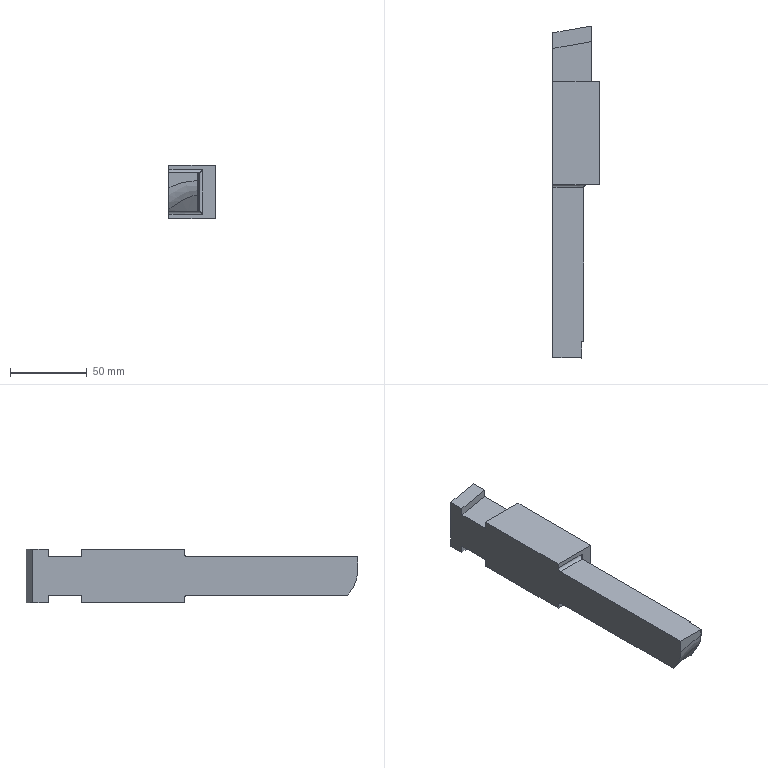Part | STEP file | solid 33 | 1 solid | 32 faces | box 30 x 215.791 x 35 mm | volume 148988 mm3 | plane 20 | cylinder 6 | spline 5 | torus 1 | commonest cylinder face diameters 4 x3 0.502 x1 1.005 x1 6.03 x1